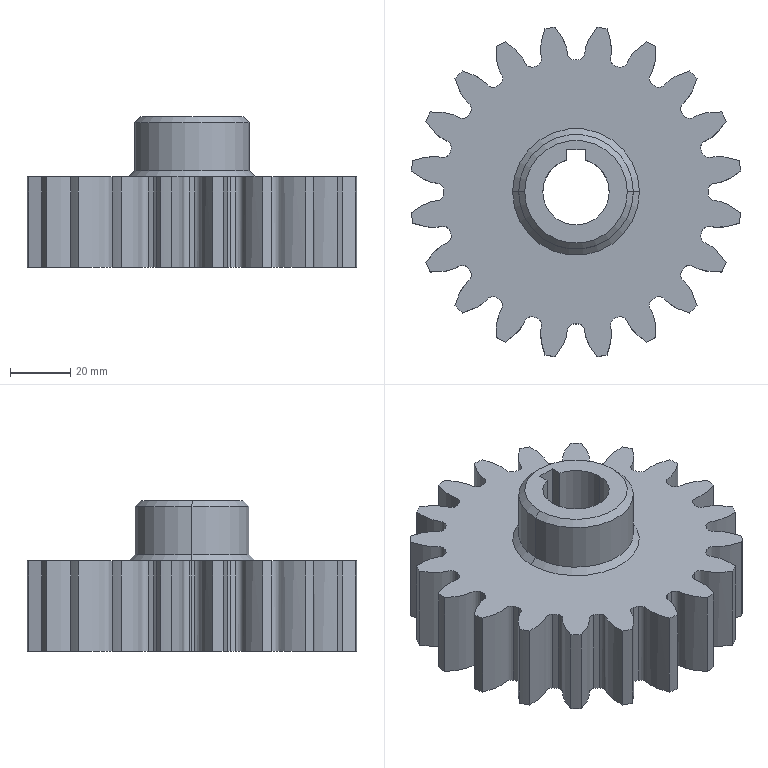Part | SolidWorks | features ICE 3, Chamfer 1, CirPattern 1, Extrusion 1, RefAxis 1 | 1 solid | 96 faces | box 109.134 x 109.134 x 50 mm | volume 234157 mm3 | cylinder 46 | spline 40 | plane 6 | cone 4 | commonest cylinder face diameters 87.5 x21 110 x20 22 x3 38 x2